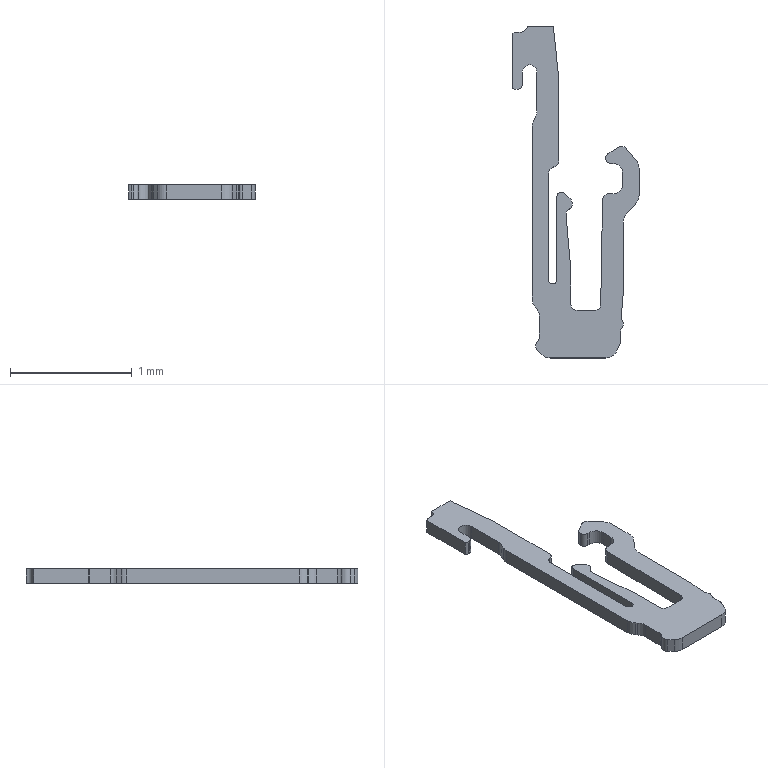Part | Creo | 1 solid | 74 faces | box 1.038 x 2.73 x 0.12 mm | volume 0.1282 mm3 | plane 39 | cylinder 35 | commonest cylinder face diameters 0.1 x16 0.2 x9 0.08 x4 0.07 x2 0.16 x2 0.099 x1